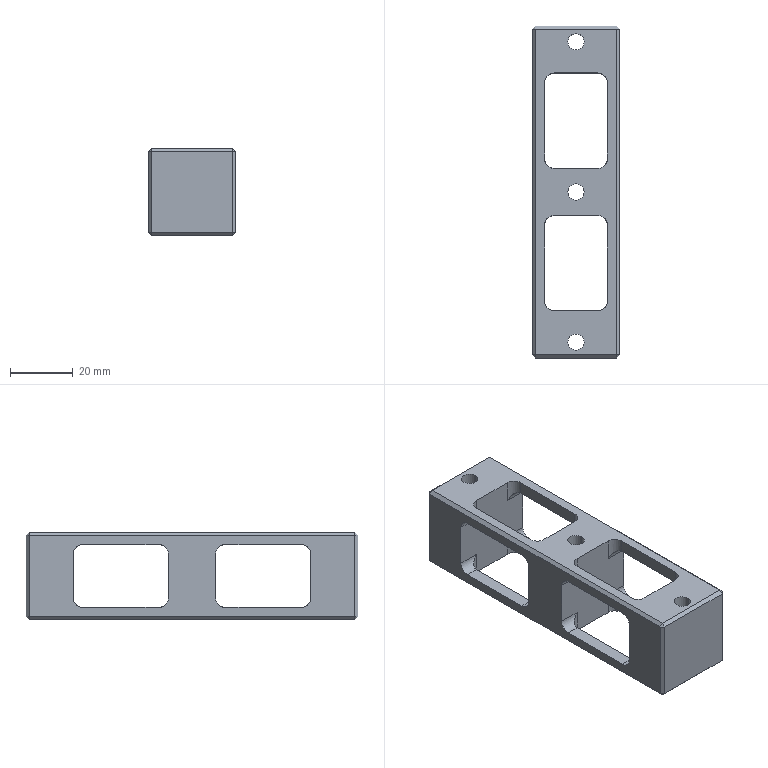Part | SolidWorks | features ICE 2, Chamfer 1, Extrusion 1 | 1 solid | 84 faces | box 28 x 106 x 28 mm | volume 37370 mm3 | plane 46 | cylinder 38 | commonest cylinder face diameters 6 x32 5.2 x6